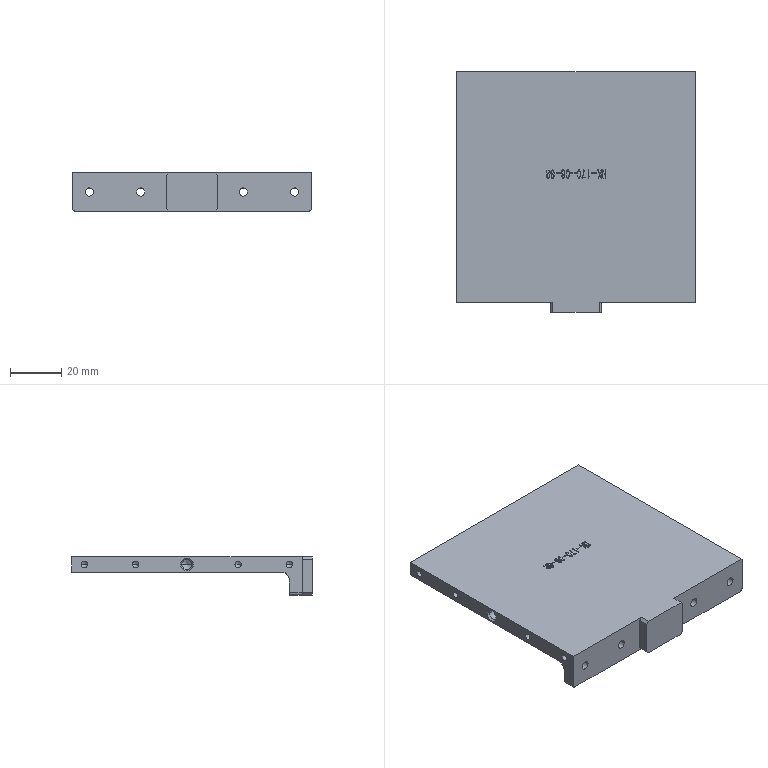NC program | NX | posted with a generic post | part box 93.2 x 94 x 15 mm
Lines 2301 to 2664 of 2664:
(PLANAR_MILL_COPY_COPY_COPY_COPY_COPY , TOOL : D6A45)
N4600 T01 M6
N4602 G54
N4604 G17 G0 G90 X-48. Y1.134 B0. C0. S9500 M3
N4606 G43 Z30. H1
N4608 Z0.5
N4610 G94 G1 Z-1. F1250.
N4612 G3 X-47.5 Y2. R1.
N4614 G1 Y47.
N4616 G2 X-46.6 Y47.9 R0.9
N4618 G1 X46.6
N4620 G2 X47.5 Y47. R0.9
N4622 G1 Y-43.
N4624 G2 X46.6 Y-43.9 R0.9
N4626 G1 X10.9
N4628 Y-47.
N4630 G2 X10. Y-47.9 R0.9
N4632 G1 X-10.
N4634 G2 X-10.9 Y-47. R0.9
N4636 G1 Y-43.9
N4638 X-46.6
N4640 G2 X-47.5 Y-43. R0.9
N4642 G1 Y2.
N4644 G3 X-48. Y2.866 R1.
N4646 G1 Z0.5
N4648 G0 Z30.
N4650 M5
(ZLEVEL_PROFILE_COPY_1_COPY_COPY_1 , TOOL : D10JING)
N4652 T14 M6
N4654 G54
N4656 G17 G0 G90 X-53.409 Y-44.622 B0. C0. S9500 M3
N4658 G43 Z30. H14
N4660 Z-13.525
N4662 G94 G1 Z-14.525 F1000.
N4664 X-52.1 Y-43.866
N4666 G3 X-51.6 Y-43. R1.
N4668 G1 Y47. F1200.
N4670 G2 X-46.6 Y52. R5.
N4672 G1 X46.6
N4674 G2 X51.6 Y47. R5.
N4676 G1 Y-43.
N4678 G2 X46.6 Y-48. R5.
N4680 G1 X14.899
N4682 G2 X10. Y-52. R5.
N4684 G1 X-10.
N4686 G2 X-14.899 Y-48. R5.
N4688 G1 X-46.6
N4690 G2 X-51.6 Y-43. R5.
N4692 G1 Y47. Z-14.553
N4694 X-51.576 Y47.49
N4696 X-51.504 Y47.975
N4698 X-51.385 Y48.451
N4700 X-51.219 Y48.913 Z-14.554
N4702 X-51.01 Y49.357
N4704 X-50.757 Y49.778
N4706 X-50.465 Y50.172
N4708 X-50.136 Y50.536
N4710 X-49.772 Y50.865
N4712 X-49.378 Y51.157 Z-14.555
N4714 X-48.957 Y51.41
N4716 X-48.513 Y51.619
N4718 X-48.051 Y51.785
N4720 X-47.575 Y51.904
N4722 X-47.09 Y51.976
N4724 X-46.6 Y52.
N4726 X46.6 Z-14.584
N4728 X47.09 Y51.976 Z-14.585
N4730 X47.575 Y51.904
N4732 X48.051 Y51.785
N4734 X48.513 Y51.619
N4736 X48.957 Y51.41
N4738 X49.378 Y51.157
N4740 X49.772 Y50.865 Z-14.586
N4742 X50.136 Y50.536
N4744 X50.465 Y50.172
N4746 X50.757 Y49.778
N4748 X51.01 Y49.357
N4750 X51.219 Y48.913
N4752 X51.385 Y48.451
N4754 X51.504 Y47.975 Z-14.587
N4756 X51.576 Y47.49
N4758 X51.6 Y47.
N4760 Y-43. Z-14.615
N4762 X51.576 Y-43.49
N4764 X51.504 Y-43.975
N4766 X51.385 Y-44.451
N4768 X51.219 Y-44.913 Z-14.616
N4770 X51.01 Y-45.357
N4772 X50.757 Y-45.778
N4774 X50.465 Y-46.172
N4776 X50.136 Y-46.536
N4778 X49.772 Y-46.865
N4780 X49.378 Y-47.157
N4782 X48.957 Y-47.41 Z-14.617
N4784 X48.513 Y-47.619
N4786 X48.051 Y-47.785
N4788 X47.575 Y-47.904
N4790 X47.09 Y-47.976
N4792 X46.6 Y-48.
N4794 X14.899 Z-14.627
N4796 X14.775 Y-48.482
N4798 X14.611 Y-48.933 Z-14.628
N4800 X14.4 Y-49.374
N4802 X14.147 Y-49.793
N4804 X13.855 Y-50.184
N4806 X13.525 Y-50.546
N4808 X13.162 Y-50.873
N4810 X12.769 Y-51.163
N4812 X12.349 Y-51.414 Z-14.629
N4814 X11.907 Y-51.622
N4816 X11.446 Y-51.786
N4818 X10.972 Y-51.905
N4820 X10.488 Y-51.976
N4822 X10. Y-52.
N4824 X-10. Z-14.636
N4826 X-10.488 Y-51.976
N4828 X-10.972 Y-51.905
N4830 X-11.446 Y-51.786
N4832 X-11.907 Y-51.622
N4834 X-12.349 Y-51.414
N4836 X-12.769 Y-51.163
N4838 X-13.162 Y-50.873 Z-14.637
N4840 X-13.525 Y-50.546
N4842 X-13.855 Y-50.184
N4844 X-14.147 Y-49.793
N4846 X-14.4 Y-49.374
N4848 X-14.611 Y-48.933
N4850 X-14.775 Y-48.482 Z-14.638
N4852 X-14.899 Y-48.
N4854 X-46.6 Z-14.648
N4856 X-47.09 Y-47.976
N4858 X-47.575 Y-47.904
N4860 X-48.051 Y-47.785
N4862 X-48.513 Y-47.619
N4864 X-48.957 Y-47.41
N4866 X-49.378 Y-47.157
N4868 X-49.772 Y-46.865 Z-14.649
N4870 X-50.136 Y-46.536
N4872 X-50.465 Y-46.172
N4874 X-50.757 Y-45.778
N4876 X-51.01 Y-45.357
N4878 X-51.219 Y-44.913
N4880 X-51.385 Y-44.451 Z-14.65
N4882 X-51.504 Y-43.975
N4884 X-51.576 Y-43.49
N4886 X-51.6 Y-43.
N4888 Y47. Z-14.678
N4890 X-51.576 Y47.49
N4892 X-51.504 Y47.975
N4894 X-51.385 Y48.451
N4896 X-51.219 Y48.913 Z-14.679
N4898 X-51.01 Y49.357
N4900 X-50.757 Y49.778
N4902 X-50.465 Y50.172
N4904 X-50.136 Y50.536
N4906 X-49.772 Y50.865
N4908 X-49.378 Y51.157 Z-14.68
N4910 X-48.957 Y51.41
N4912 X-48.513 Y51.619
N4914 X-48.051 Y51.785
N4916 X-47.575 Y51.904
N4918 X-47.09 Y51.976
N4920 X-46.6 Y52.
N4922 X46.6 Z-14.709
N4924 X47.09 Y51.976 Z-14.71
N4926 X47.575 Y51.904
N4928 X48.051 Y51.785
N4930 X48.513 Y51.619
N4932 X48.957 Y51.41
N4934 X49.378 Y51.157
N4936 X49.772 Y50.865 Z-14.711
N4938 X50.136 Y50.536
N4940 X50.465 Y50.172
N4942 X50.757 Y49.778
N4944 X51.01 Y49.357
N4946 X51.219 Y48.913
N4948 X51.385 Y48.451
N4950 X51.504 Y47.975 Z-14.712
N4952 X51.576 Y47.49
N4954 X51.6 Y47.
N4956 Y-43. Z-14.74
N4958 X51.576 Y-43.49
N4960 X51.504 Y-43.975
N4962 X51.385 Y-44.451
N4964 X51.219 Y-44.913 Z-14.741
N4966 X51.01 Y-45.357
N4968 X50.757 Y-45.778
N4970 X50.465 Y-46.172
N4972 X50.136 Y-46.536
N4974 X49.772 Y-46.865
N4976 X49.378 Y-47.157
N4978 X48.957 Y-47.41 Z-14.742
N4980 X48.513 Y-47.619
N4982 X48.051 Y-47.785
N4984 X47.575 Y-47.904
N4986 X47.09 Y-47.976
N4988 X46.6 Y-48.
N4990 X14.899 Z-14.752
N4992 X14.775 Y-48.482
N4994 X14.611 Y-48.933 Z-14.753
N4996 X14.4 Y-49.374
N4998 X14.147 Y-49.793
N5000 X13.855 Y-50.184
N5002 X13.525 Y-50.546
N5004 X13.162 Y-50.873
N5006 X12.769 Y-51.163
N5008 X12.349 Y-51.414 Z-14.754
N5010 X11.907 Y-51.622
N5012 X11.446 Y-51.786
N5014 X10.972 Y-51.905
N5016 X10.488 Y-51.976
N5018 X10. Y-52.
N5020 X-10. Z-14.761
N5022 X-10.488 Y-51.976
N5024 X-10.972 Y-51.905
N5026 X-11.446 Y-51.786
N5028 X-11.907 Y-51.622
N5030 X-12.349 Y-51.414
N5032 X-12.769 Y-51.163
N5034 X-13.162 Y-50.873 Z-14.762
N5036 X-13.525 Y-50.546
N5038 X-13.855 Y-50.184
N5040 X-14.147 Y-49.793
N5042 X-14.4 Y-49.374
N5044 X-14.611 Y-48.933
N5046 X-14.775 Y-48.482 Z-14.763
N5048 X-14.899 Y-48.
N5050 X-46.6 Z-14.773
N5052 X-47.09 Y-47.976
N5054 X-47.575 Y-47.904
N5056 X-48.051 Y-47.785
N5058 X-48.513 Y-47.619
N5060 X-48.957 Y-47.41
N5062 X-49.378 Y-47.157
N5064 X-49.772 Y-46.865 Z-14.774
N5066 X-50.136 Y-46.536
N5068 X-50.465 Y-46.172
N5070 X-50.757 Y-45.778
N5072 X-51.01 Y-45.357
N5074 X-51.219 Y-44.913
N5076 X-51.385 Y-44.451 Z-14.775
N5078 X-51.504 Y-43.975
N5080 X-51.576 Y-43.49
N5082 X-51.6 Y-43.
N5084 Y47. Z-14.803
N5086 X-51.576 Y47.49
N5088 X-51.504 Y47.975
N5090 X-51.385 Y48.451
N5092 X-51.219 Y48.913 Z-14.804
N5094 X-51.01 Y49.357
N5096 X-50.757 Y49.778
N5098 X-50.465 Y50.172
N5100 X-50.136 Y50.536
N5102 X-49.772 Y50.865
N5104 X-49.378 Y51.157 Z-14.805
N5106 X-48.957 Y51.41
N5108 X-48.513 Y51.619
N5110 X-48.051 Y51.785
N5112 X-47.575 Y51.904
N5114 X-47.09 Y51.976
N5116 X-46.6 Y52.
N5118 X46.6 Z-14.834
N5120 X47.09 Y51.976 Z-14.835
N5122 X47.575 Y51.904
N5124 X48.051 Y51.785
N5126 X48.513 Y51.619
N5128 X48.957 Y51.41
N5130 X49.378 Y51.157
N5132 X49.772 Y50.865 Z-14.836
N5134 X50.136 Y50.536
N5136 X50.465 Y50.172
N5138 X50.757 Y49.778
N5140 X51.01 Y49.357
N5142 X51.219 Y48.913
N5144 X51.385 Y48.451
N5146 X51.504 Y47.975 Z-14.837
N5148 X51.576 Y47.49
N5150 X51.6 Y47.
N5152 Y-43. Z-14.865
N5154 X51.576 Y-43.49
N5156 X51.504 Y-43.975
N5158 X51.385 Y-44.451
N5160 X51.219 Y-44.913 Z-14.866
N5162 X51.01 Y-45.357
N5164 X50.757 Y-45.778
N5166 X50.465 Y-46.172
N5168 X50.136 Y-46.536
N5170 X49.772 Y-46.865
N5172 X49.378 Y-47.157
N5174 X48.957 Y-47.41 Z-14.867
N5176 X48.513 Y-47.619
N5178 X48.051 Y-47.785
N5180 X47.575 Y-47.904
N5182 X47.09 Y-47.976
N5184 X46.6 Y-48.
N5186 X14.899 Z-14.877
N5188 X14.775 Y-48.482
N5190 X14.611 Y-48.933 Z-14.878
N5192 X14.4 Y-49.374
N5194 X14.147 Y-49.793
N5196 X13.855 Y-50.184
N5198 X13.525 Y-50.546
N5200 X13.162 Y-50.873
N5202 X12.769 Y-51.163
N5204 X12.349 Y-51.414 Z-14.879
N5206 X11.907 Y-51.622
N5208 X11.446 Y-51.786
N5210 X10.972 Y-51.905
N5212 X10.488 Y-51.976
N5214 X10. Y-52.
N5216 X-10. Z-14.886
N5218 X-10.488 Y-51.976
N5220 X-10.972 Y-51.905
N5222 X-11.446 Y-51.786
N5224 X-11.907 Y-51.622
N5226 X-12.349 Y-51.414
N5228 X-12.769 Y-51.163
N5230 X-13.162 Y-50.873 Z-14.887
N5232 X-13.525 Y-50.546
N5234 X-13.855 Y-50.184
N5236 X-14.147 Y-49.793
N5238 X-14.4 Y-49.374
N5240 X-14.611 Y-48.933
N5242 X-14.775 Y-48.482 Z-14.888
N5244 X-14.899 Y-48.
N5246 X-46.6 Z-14.898
N5248 X-47.09 Y-47.976
N5250 X-47.575 Y-47.904
N5252 X-48.051 Y-47.785
N5254 X-48.513 Y-47.619
N5256 X-48.957 Y-47.41
N5258 X-49.378 Y-47.157
N5260 X-49.772 Y-46.865 Z-14.899
N5262 X-50.136 Y-46.536
N5264 X-50.465 Y-46.172
N5266 X-50.757 Y-45.778
N5268 X-51.01 Y-45.357
N5270 X-51.219 Y-44.913
N5272 X-51.385 Y-44.451 Z-14.9
N5274 X-51.504 Y-43.975
N5276 X-51.576 Y-43.49
N5278 X-51.6 Y-43.
N5280 Y47.
N5282 G2 X-46.6 Y52. R5.
N5284 G1 X46.6
N5286 G2 X51.6 Y47. R5.
N5288 G1 Y-43.
N5290 G2 X46.6 Y-48. R5.
N5292 G1 X14.899
N5294 G2 X10. Y-52. R5.
N5296 G1 X-10.
N5298 G2 X-14.899 Y-48. R5.
N5300 G1 X-46.6
N5302 G2 X-51.6 Y-43. R5.
N5304 G3 X-52.1 Y-42.134 R1.
N5306 G1 X-53.6 Y-41.268
N5308 Z-13.9
N5310 G0 Z30.
N5312 M5
N5314 M2